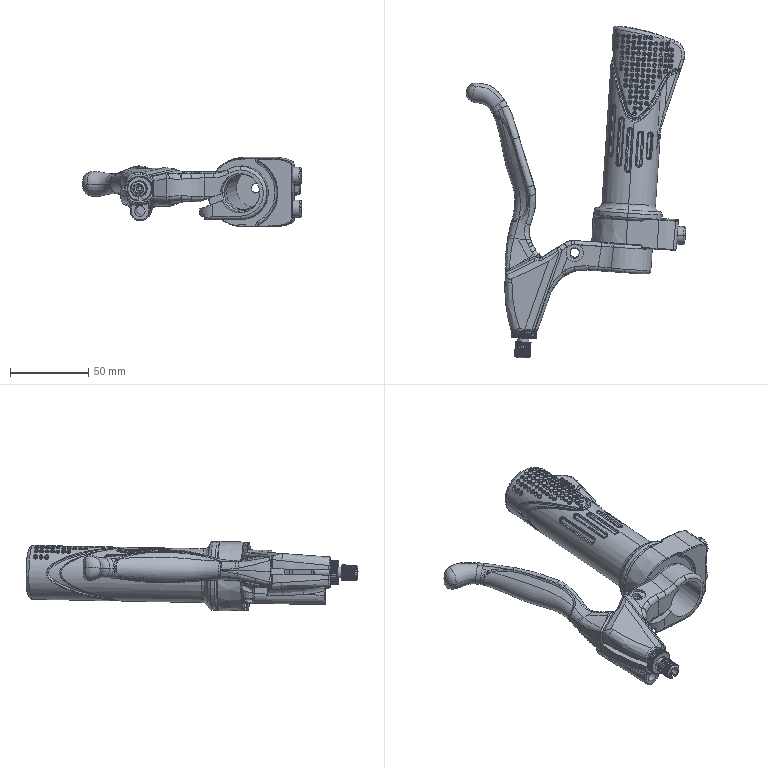Part | SolidWorks | features BaseBody 1 | 1 solid | 1864 faces | box 140.406 x 212.588 x 44.525 mm | volume 142140 mm3 | spline 892 | cylinder 650 | plane 196 | cone 63 | torus 56 | sphere 7 | commonest cylinder face diameters 2 x131 32.5 x114 0.6 x91 16 x34 2.24 x32 1.12 x30